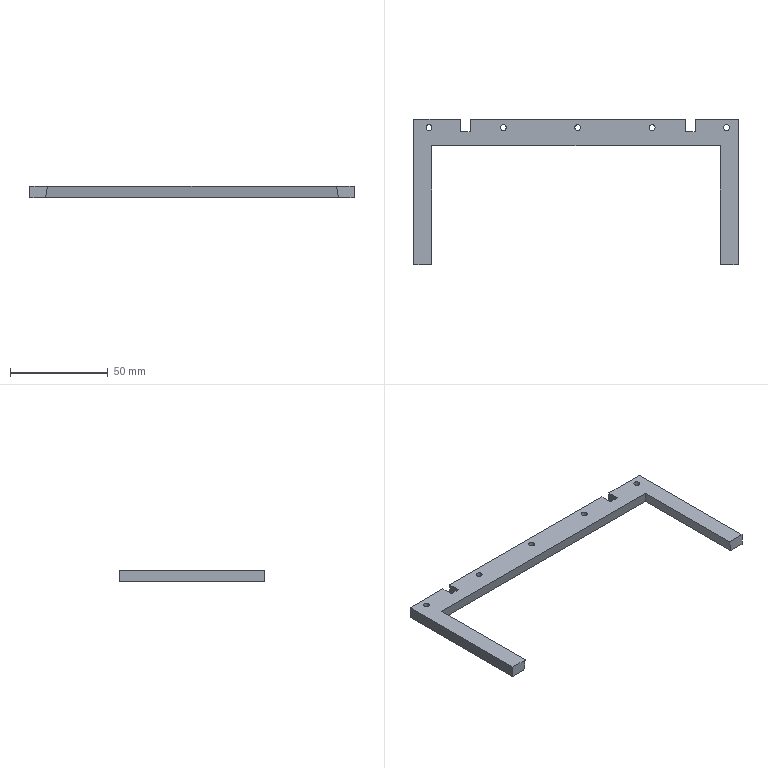Part | STEP file | 1-56.18 | 1 solid | 23 faces | box 165.767 x 74.2 x 6 mm | volume 18558 mm3 | plane 18 | cylinder 5 | commonest cylinder face diameters 3 x5